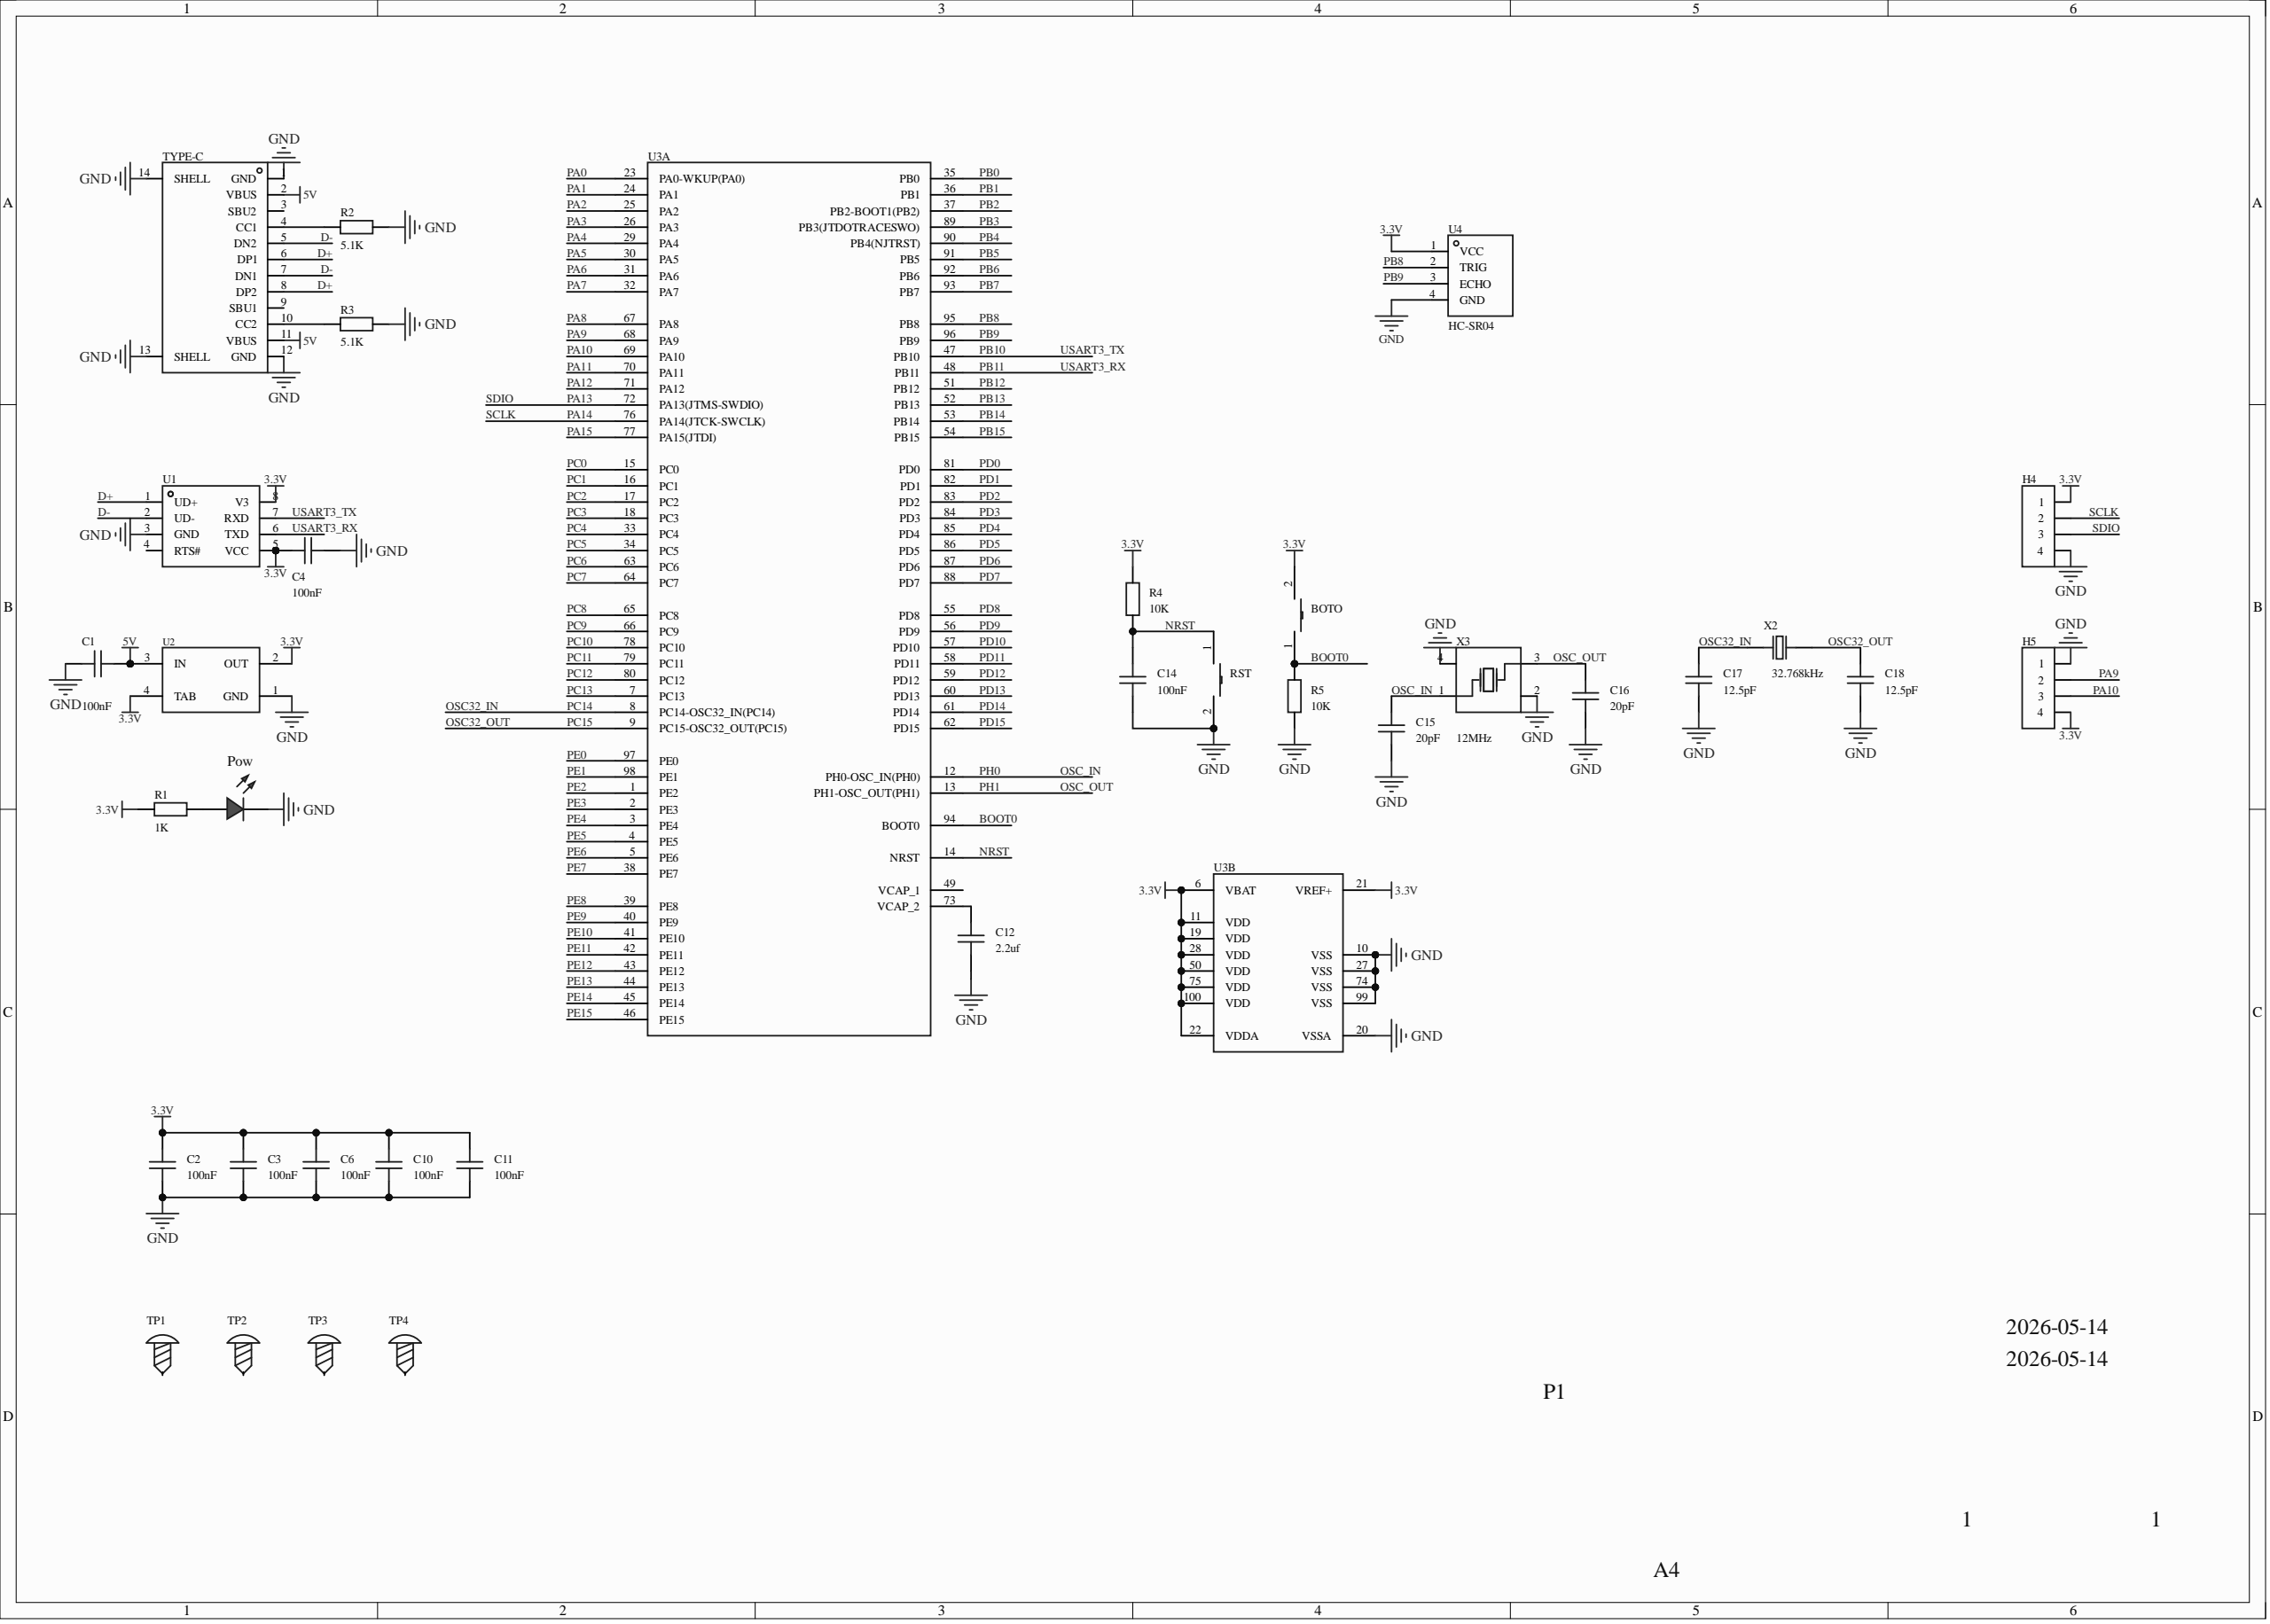Circuit board | Altium Designer | 34 parts | 23 nets
Bill of materials:
Comment,Description,Designator,Footprint,LibRef,Quantity
"TS-1101-C-W","Contact current: 50mA; rated voltage (AC): -; rated voltage (DC): 12V; rated power: -; insulation resistance: -; circuit structure: SPST; mounting: SMD vertical; with lamp: no; actuating force: 260gf; mechanical life: 5万 cycles; with bracket: no;","BOTO, RST","SW-SMD_L6.0-W3.3-LS8.0","TS-1101-C-W","2"
"CAP_0603","","C1, C2, C3, C4, C6, C10, C11, C12, C14, C15, C16, C17, C18","C0603","CAP_0603","13"
"Side-solder 1X4 pin header","","H4, H5","侧焊1X4排针","侧焊1X4排针","2"
"LED_0603-R","","Pow","LED_0603","LED_0603-R","1"
"Res_0603","","R1, R2, R3, R4, R5","R0603","Res_0603","5"
"M3 screw","","TP1, TP2, TP3, TP4","M3螺丝","M3螺丝","4"
"TYPE-C 16PIN 2MD(073)","Connector type: Type-C; standard: -; gender: female; contact count: 16P; port count: 1; mounting: SMD horizontal; rated current - power: 5A; operating temperature: -25℃~+85℃;","TYPE-C","USB-C-SMD_TYPE-C-6PIN-2MD-073","TYPE-C 16PIN 2MD(073)","1"
"CH340N","","U1","SOP-8_L4.9-W3.9-P1.27-LS6.0-BL","CH340N","1"
"LM1117IMPX-3.3/NOPB","Output type: fixed; output polarity: positive; max input voltage: 15V; output voltage: 3.3V; output current: 800mA; ripple rejection (PSRR): 75dB@(120Hz);","U2","SOT-223_L6.5-W3.5-P2.30-LS7.0-BR","LM1117IMPX-3.3/NOPB","1"
"","CPU core: ARM Cortex-M4; max CPU frequency: 168MHz; operating voltage: 1.8V~3.6V; internal oscillator: yes; program FLASH: 512K@x8bit; total RAM: 192KB; EEPROM/data FLASH: -; GPIO ports: 82; ADC (units/channels/bits): 1@x16ch/12bit; DAC (units/channels/bits): 1@x2ch/12bit; peripherals/functions/protocol stacks: undervoltage detection/reset; DMA; LCD driver; watchdog; POR; PWM; operating temperature: -40℃~+85℃;","U3","LQFP-100_L14.0-W14.0-P0.50-LS16.0-BL","STM32F407VET6","1"
"HC-SR04","","U4","TH_HC-SR04V","HC-SR04","1"
"Q13FC1350000400","Frequency: 32.768kHz; frequency tolerance: ±20ppm; load capacitance: 12.5pF;","X2","FC-135R_L3.2-W1.5","Q13FC1350000400","1"
"X322512MSB4SI","Crystal type: SMD crystal; frequency: 12MHz; frequency tolerance (room temp): ±10ppm; external load capacitance: 20pF; frequency stability (full temp): ±30ppm;","X3","OSC-SMD_4P-L3.2-W2.5-BL","X322512MSB4SI","1"
Netlist (Protel format):
[
BOTO
SW-SMD_L6.0-W3.3-LS8.0
TS-1101-C-W



]
[
C1
C0603
CAP_0603



]
[
C2
C0603
CAP_0603



]
[
C3
C0603
CAP_0603



]
[
C4
C0603
CAP_0603



]
[
C6
C0603
CAP_0603



]
[
C10
C0603
CAP_0603



]
[
C11
C0603
CAP_0603



]
[
C12
C0603
CAP_0603



]
[
C14
C0603
CAP_0603



]
[
C15
C0603
CAP_0603



]
[
C16
C0603
CAP_0603



]
[
C17
C0603
CAP_0603



]
[
C18
C0603
CAP_0603



]
[
H4
侧焊1X4排针
Side-solder 1X4 pin header



]
[
H5
侧焊1X4排针
Side-solder 1X4 pin header



]
[
Pow
LED_0603
LED_0603-R



]
[
R1
R0603
Res_0603



]
[
R2
R0603
Res_0603



]
[
R3
R0603
Res_0603



]
[
R4
R0603
Res_0603



]
[
R5
R0603
Res_0603



]
[
RST
SW-SMD_L6.0-W3.3-LS8.0
TS-1101-C-W



]
[
TP1
M3螺丝
M3 screw



]
[
TP2
M3螺丝
M3 screw



]
[
TP3
M3螺丝
M3 screw



]
[
TP4
M3螺丝
M3 screw



]
[
TYPE-C
USB-C-SMD_TYPE-C-6PIN-2MD-073
TYPE-C 16PIN 2MD(073)



]
[
U1
SOP-8_L4.9-W3.9-P1.27-LS6.0-BL
CH340N



]
[
U2
SOT-223_L6.5-W3.5-P2.30-LS7.0-BR
LM1117IMPX-3.3/NOPB



]
[
U3
LQFP-100_L14.0-W14.0-P0.50-LS16.0-BL




]
[
U4
TH_HC-SR04V
HC-SR04



]
[
X2
FC-135R_L3.2-W1.5
Q13FC1350000400



]
[
X3
OSC-SMD_4P-L3.2-W2.5-BL
X322512MSB4SI



]
(
PB11
U1-6
U3-48
)
(
PB10
U1-7
U3-47
)
(
PB9
U3-96
U4-3
)
(
PB8
U3-95
U4-2
)
(
PA14
H4-2
U3-76
)
(
PA13
H4-3
U3-72
)
(
PA10
H5-3
U3-69
)
(
PA9
H5-2
U3-68
)
(
OSC_OUT
C16-2
U3-13
X3-3
)
(
OSC_IN
C15-2
U3-12
X3-1
)
(
OSC32_OUT
C18-2
U3-9
X2-2
)
(
OSC32_IN
C17-2
U3-8
X2-1
)
(
NRST
C14-2
R4-1
RST-1
U3-14
)
(
NetR3_2
R3-2
TYPE-C-10
)
(
NetR2_2
R2-2
TYPE-C-4
)
(
NetPow_2
Pow-2
R1-2
)
(
NetC12_1
C12-1
U3-73
)
(
GND
C1-1
C2-1
C3-1
C4-2
C6-1
C10-1
C11-1
C12-2
C14-1
C15-1
C16-1
C17-1
C18-1
H4-4
H5-1
Pow-1
R2-1
R3-1
R5-1
RST-2
TYPE-C-1
TYPE-C-12
TYPE-C-13
TYPE-C-14
U1-3
U2-1
U3-10
U3-20
U3-27
U3-74
U3-99
U4-4
X3-2
X3-4
)
(
D-
TYPE-C-5
TYPE-C-7
U1-2
)
(
D+
TYPE-C-6
TYPE-C-8
U1-1
)
(
BOOT0
BOTO-1
R5-2
U3-94
)
(
5V
C1-2
TYPE-C-2
TYPE-C-11
U2-3
)
(
3.3V
BOTO-2
C2-2
C3-2
C4-1
C6-2
C10-2
C11-2
H4-1
H5-4
R1-1
R4-2
U1-5
U1-8
U2-2
U2-4
U3-6
U3-11
U3-19
U3-21
U3-22
U3-28
U3-50
U3-75
U3-100
U4-1
)